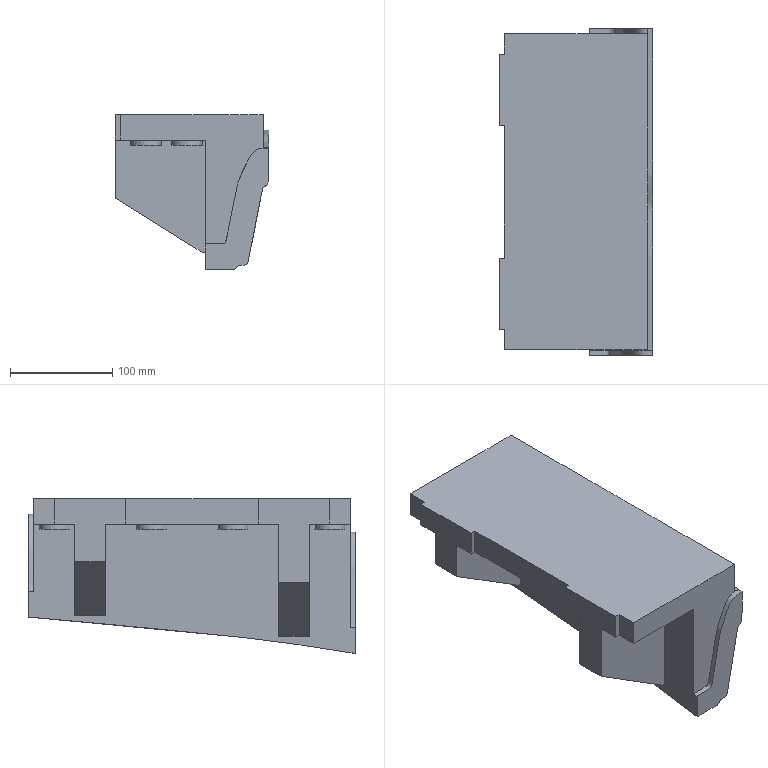Part | NX | features solid 2 | 1 solid | 115 faces | box 150.316 x 320 x 151.842 mm | volume 3331860 mm3 | spline 65 | plane 32 | cylinder 18 | commonest cylinder face diameters 30 x6 6.001 x3 10.001 x2 5.989 x1 9.006 x1 9.989 x1